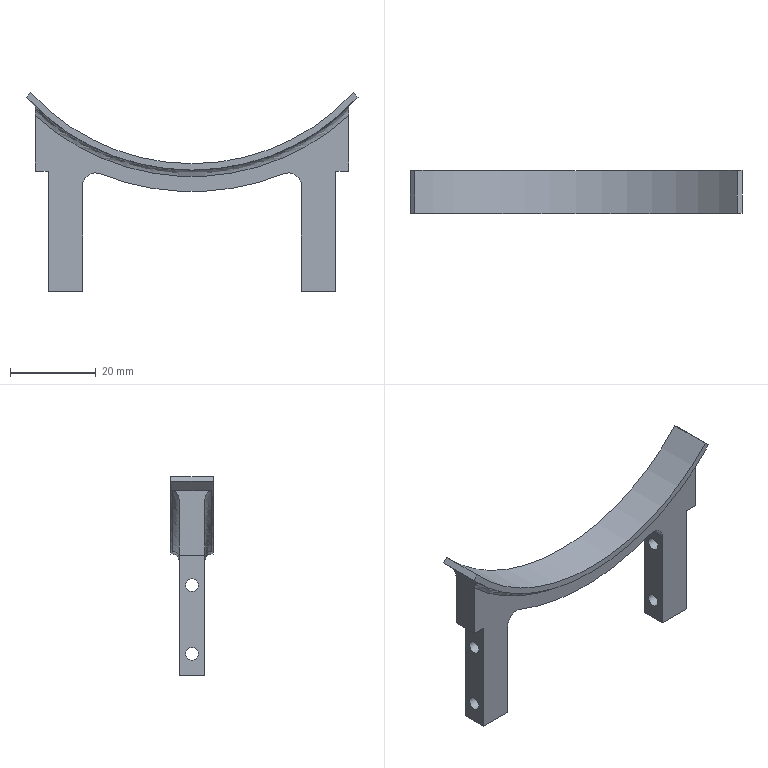Part | STEP file | 1-59 | 1 solid | 27 faces | box 77.36 x 10 x 46.251 mm | volume 6866 mm3 | plane 16 | cylinder 9 | spline 2 | commonest cylinder face diameters 3 x4 6 x2 102 x1 105 x1 115 x1